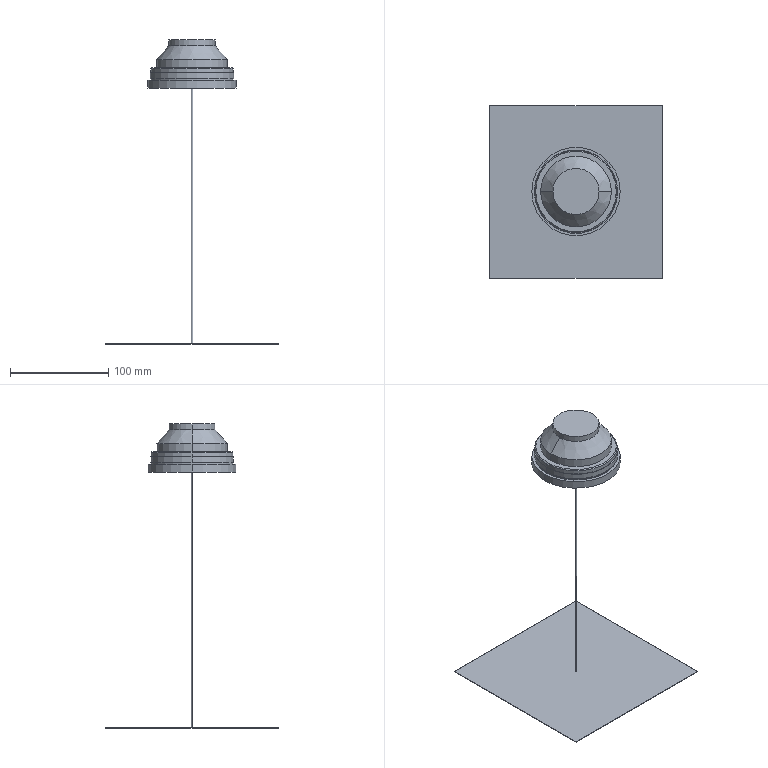Part | SolidWorks | features ICE 8, Draft 3, Chamfer 2, Extrusion 1, RevCut 1 | 1 solid | 30 faces | box 175 x 175 x 309.5 mm | volume 221478 mm3 | cylinder 14 | plane 12 | cone 4 | commonest cylinder face diameters 84 x4 2 x2 47 x2 72 x2 85 x2 90 x2
STEP:
#1=CARTESIAN_POINT('',(-1.,0.,-260.));
#2=VERTEX_POINT('',#1);
#3=CARTESIAN_POINT('',(1.,0.,-260.));
#4=VERTEX_POINT('',#3);
#5=CARTESIAN_POINT('',(0.,0.,-260.));
#6=DIRECTION('',(0.,0.,-1.));
#7=DIRECTION('',(-1.,0.,0.));
#8=AXIS2_PLACEMENT_3D('',#5,#6,#7);
#9=CIRCLE('',#8,1.);
#10=EDGE_CURVE('',#2,#4,#9,.T.);
#11=ORIENTED_EDGE('',*,*,#10,.F.);
#12=CARTESIAN_POINT('',(-1.,0.,0.));
#13=VERTEX_POINT('',#12);
#14=CARTESIAN_POINT('',(-1.,0.,-260.));
#15=DIRECTION('',(0.,0.,1.));
#16=VECTOR('',#15,1000.);
#17=LINE('',#14,#16);
#18=EDGE_CURVE('',#2,#13,#17,.T.);
#19=ORIENTED_EDGE('',*,*,#18,.T.);
#20=CARTESIAN_POINT('',(1.,0.,0.));
#21=VERTEX_POINT('',#20);
#22=CARTESIAN_POINT('',(0.,0.,0.));
#23=DIRECTION('',(0.,0.,-1.));
#24=DIRECTION('',(1.,0.,0.));
#25=AXIS2_PLACEMENT_3D('',#22,#23,#24);
#26=CIRCLE('',#25,1.);
#27=EDGE_CURVE('',#13,#21,#26,.T.);
#28=ORIENTED_EDGE('',*,*,#27,.T.);
#29=CARTESIAN_POINT('',(1.,0.,-260.));
#30=DIRECTION('',(0.,0.,1.));
#31=VECTOR('',#30,1000.);
#32=LINE('',#29,#31);
#33=EDGE_CURVE('',#4,#21,#32,.T.);
#34=ORIENTED_EDGE('',*,*,#33,.F.);
#35=EDGE_LOOP('',(#11,#19,#28,#34));
#36=FACE_OUTER_BOUND('',#35,.T.);
#37=CARTESIAN_POINT('',(0.,0.,-260.));
#38=DIRECTION('',(0.,0.,1.));
#39=DIRECTION('',(1.,0.,0.));
#40=AXIS2_PLACEMENT_3D('',#37,#38,#39);
#41=CYLINDRICAL_SURFACE('',#40,1.);
#42=ADVANCED_FACE('',(#36),#41,.T.);
#43=CARTESIAN_POINT('',(41.,0.,20.5));
#44=VERTEX_POINT('',#43);
#45=CARTESIAN_POINT('',(-41.,0.,20.5));
#46=VERTEX_POINT('',#45);
#47=CARTESIAN_POINT('',(0.,0.,20.5));
#48=DIRECTION('',(0.,0.,1.));
#49=DIRECTION('',(1.,0.,0.));
#50=AXIS2_PLACEMENT_3D('',#47,#48,#49);
#51=CIRCLE('',#50,41.);
#52=EDGE_CURVE('',#44,#46,#51,.T.);
#53=ORIENTED_EDGE('',*,*,#52,.F.);
#54=CARTESIAN_POINT('',(42.,0.,19.5));
#55=VERTEX_POINT('',#54);
#56=CARTESIAN_POINT('',(42.,0.,19.5));
#57=DIRECTION('',(0.7071,0.,-0.7071));
#58=VECTOR('',#57,1000.);
#59=LINE('',#56,#58);
#60=EDGE_CURVE('',#44,#55,#59,.T.);
#61=ORIENTED_EDGE('',*,*,#60,.T.);
#62=CARTESIAN_POINT('',(-42.,0.,19.5));
#63=VERTEX_POINT('',#62);
#64=CARTESIAN_POINT('',(0.,0.,19.5));
#65=DIRECTION('',(0.,0.,-1.));
#66=DIRECTION('',(1.,0.,0.));
#67=AXIS2_PLACEMENT_3D('',#64,#65,#66);
#68=CIRCLE('',#67,42.);
#69=EDGE_CURVE('',#63,#55,#68,.T.);
#70=ORIENTED_EDGE('',*,*,#69,.F.);
#71=CARTESIAN_POINT('',(-42.,0.,19.5));
#72=DIRECTION('',(-0.7071,0.,-0.7071));
#73=VECTOR('',#72,1000.);
#74=LINE('',#71,#73);
#75=EDGE_CURVE('',#46,#63,#74,.T.);
#76=ORIENTED_EDGE('',*,*,#75,.F.);
#77=EDGE_LOOP('',(#53,#61,#70,#76));
#78=FACE_OUTER_BOUND('',#77,.T.);
#79=CARTESIAN_POINT('',(0.,0.,19.5));
#80=DIRECTION('',(0.,0.,-1.));
#81=DIRECTION('',(-1.,0.,0.));
#82=AXIS2_PLACEMENT_3D('',#79,#80,#81);
#83=CONICAL_SURFACE('',#82,42.,0.7854);
#84=ADVANCED_FACE('',(#78),#83,.T.);
#85=CARTESIAN_POINT('',(36.,0.,29.));
#86=VERTEX_POINT('',#85);
#87=CARTESIAN_POINT('',(-36.,0.,29.));
#88=VERTEX_POINT('',#87);
#89=CARTESIAN_POINT('',(0.,0.,29.));
#90=DIRECTION('',(0.,0.,1.));
#91=DIRECTION('',(1.,0.,0.));
#92=AXIS2_PLACEMENT_3D('',#89,#90,#91);
#93=CIRCLE('',#92,36.);
#94=EDGE_CURVE('',#86,#88,#93,.T.);
#95=ORIENTED_EDGE('',*,*,#94,.F.);
#96=CARTESIAN_POINT('',(36.,0.,20.5));
#97=VERTEX_POINT('',#96);
#98=CARTESIAN_POINT('',(36.,0.,29.));
#99=DIRECTION('',(0.,0.,-1.));
#100=VECTOR('',#99,1000.);
#101=LINE('',#98,#100);
#102=EDGE_CURVE('',#86,#97,#101,.T.);
#103=ORIENTED_EDGE('',*,*,#102,.T.);
#104=CARTESIAN_POINT('',(-36.,0.,20.5));
#105=VERTEX_POINT('',#104);
#106=CARTESIAN_POINT('',(0.,0.,20.5));
#107=DIRECTION('',(0.,0.,1.));
#108=DIRECTION('',(1.,0.,0.));
#109=AXIS2_PLACEMENT_3D('',#106,#107,#108);
#110=CIRCLE('',#109,36.);
#111=EDGE_CURVE('',#97,#105,#110,.T.);
#112=ORIENTED_EDGE('',*,*,#111,.T.);
#113=CARTESIAN_POINT('',(-36.,0.,29.));
#114=DIRECTION('',(0.,0.,-1.));
#115=VECTOR('',#114,1000.);
#116=LINE('',#113,#115);
#117=EDGE_CURVE('',#88,#105,#116,.T.);
#118=ORIENTED_EDGE('',*,*,#117,.F.);
#119=EDGE_LOOP('',(#95,#103,#112,#118));
#120=FACE_OUTER_BOUND('',#119,.T.);
#121=CARTESIAN_POINT('',(0.,0.,29.));
#122=DIRECTION('',(0.,0.,-1.));
#123=DIRECTION('',(-1.,0.,0.));
#124=AXIS2_PLACEMENT_3D('',#121,#122,#123);
#125=CYLINDRICAL_SURFACE('',#124,36.);
#126=ADVANCED_FACE('',(#120),#125,.T.);
#127=CARTESIAN_POINT('',(23.5,0.,43.));
#128=VERTEX_POINT('',#127);
#129=CARTESIAN_POINT('',(-23.5,0.,43.));
#130=VERTEX_POINT('',#129);
#131=CARTESIAN_POINT('',(0.,0.,43.));
#132=DIRECTION('',(0.,0.,1.));
#133=DIRECTION('',(1.,0.,0.));
#134=AXIS2_PLACEMENT_3D('',#131,#132,#133);
#135=CIRCLE('',#134,23.5);
#136=EDGE_CURVE('',#128,#130,#135,.T.);
#137=ORIENTED_EDGE('',*,*,#136,.F.);
#138=CARTESIAN_POINT('',(23.5,0.,43.));
#139=DIRECTION('',(0.666,0.,-0.7459));
#140=VECTOR('',#139,1000.);
#141=LINE('',#138,#140);
#142=EDGE_CURVE('',#128,#86,#141,.T.);
#143=ORIENTED_EDGE('',*,*,#142,.T.);
#144=ORIENTED_EDGE('',*,*,#94,.T.);
#145=CARTESIAN_POINT('',(-23.5,0.,43.));
#146=DIRECTION('',(-0.666,0.,-0.7459));
#147=VECTOR('',#146,1000.);
#148=LINE('',#145,#147);
#149=EDGE_CURVE('',#130,#88,#148,.T.);
#150=ORIENTED_EDGE('',*,*,#149,.F.);
#151=EDGE_LOOP('',(#137,#143,#144,#150));
#152=FACE_OUTER_BOUND('',#151,.T.);
#153=CARTESIAN_POINT('',(0.,0.,43.));
#154=DIRECTION('',(0.,0.,-1.));
#155=DIRECTION('',(-1.,0.,0.));
#156=AXIS2_PLACEMENT_3D('',#153,#154,#155);
#157=CONICAL_SURFACE('',#156,23.5,0.7289);
#158=ADVANCED_FACE('',(#152),#157,.T.);
#159=CARTESIAN_POINT('',(23.5,0.,49.));
#160=VERTEX_POINT('',#159);
#161=CARTESIAN_POINT('',(-23.5,0.,49.));
#162=VERTEX_POINT('',#161);
#163=CARTESIAN_POINT('',(0.,0.,49.));
#164=DIRECTION('',(0.,0.,1.));
#165=DIRECTION('',(1.,0.,0.));
#166=AXIS2_PLACEMENT_3D('',#163,#164,#165);
#167=CIRCLE('',#166,23.5);
#168=EDGE_CURVE('',#160,#162,#167,.T.);
#169=ORIENTED_EDGE('',*,*,#168,.F.);
#170=CARTESIAN_POINT('',(23.5,0.,49.));
#171=DIRECTION('',(0.,0.,-1.));
#172=VECTOR('',#171,1000.);
#173=LINE('',#170,#172);
#174=EDGE_CURVE('',#160,#128,#173,.T.);
#175=ORIENTED_EDGE('',*,*,#174,.T.);
#176=ORIENTED_EDGE('',*,*,#136,.T.);
#177=CARTESIAN_POINT('',(-23.5,0.,49.));
#178=DIRECTION('',(0.,0.,-1.));
#179=VECTOR('',#178,1000.);
#180=LINE('',#177,#179);
#181=EDGE_CURVE('',#162,#130,#180,.T.);
#182=ORIENTED_EDGE('',*,*,#181,.F.);
#183=EDGE_LOOP('',(#169,#175,#176,#182));
#184=FACE_OUTER_BOUND('',#183,.T.);
#185=CARTESIAN_POINT('',(0.,0.,49.));
#186=DIRECTION('',(0.,0.,-1.));
#187=DIRECTION('',(-1.,0.,0.));
#188=AXIS2_PLACEMENT_3D('',#185,#186,#187);
#189=CYLINDRICAL_SURFACE('',#188,23.5);
#190=ADVANCED_FACE('',(#184),#189,.T.);
#191=ORIENTED_EDGE('',*,*,#69,.T.);
#192=CARTESIAN_POINT('',(42.,0.,15.5));
#193=VERTEX_POINT('',#192);
#194=CARTESIAN_POINT('',(42.,0.,0.));
#195=DIRECTION('',(0.,0.,-1.));
#196=VECTOR('',#195,1000.);
#197=LINE('',#194,#196);
#198=EDGE_CURVE('',#55,#193,#197,.T.);
#199=ORIENTED_EDGE('',*,*,#198,.T.);
#200=CARTESIAN_POINT('',(-42.,0.,15.5));
#201=VERTEX_POINT('',#200);
#202=CARTESIAN_POINT('',(0.,0.,15.5));
#203=DIRECTION('',(0.,0.,-1.));
#204=DIRECTION('',(-1.,0.,0.));
#205=AXIS2_PLACEMENT_3D('',#202,#203,#204);
#206=CIRCLE('',#205,42.);
#207=EDGE_CURVE('',#201,#193,#206,.T.);
#208=ORIENTED_EDGE('',*,*,#207,.F.);
#209=CARTESIAN_POINT('',(-42.,0.,0.));
#210=DIRECTION('',(0.,0.,-1.));
#211=VECTOR('',#210,1000.);
#212=LINE('',#209,#211);
#213=EDGE_CURVE('',#63,#201,#212,.T.);
#214=ORIENTED_EDGE('',*,*,#213,.F.);
#215=EDGE_LOOP('',(#191,#199,#208,#214));
#216=FACE_OUTER_BOUND('',#215,.T.);
#217=CARTESIAN_POINT('',(0.,0.,0.));
#218=DIRECTION('',(0.,0.,-1.));
#219=DIRECTION('',(-1.,0.,0.));
#220=AXIS2_PLACEMENT_3D('',#217,#218,#219);
#221=CYLINDRICAL_SURFACE('',#220,42.);
#222=ADVANCED_FACE('',(#216),#221,.T.);
#223=CARTESIAN_POINT('',(45.,0.,8.));
#224=VERTEX_POINT('',#223);
#225=CARTESIAN_POINT('',(-45.,0.,8.));
#226=VERTEX_POINT('',#225);
#227=CARTESIAN_POINT('',(0.,0.,8.));
#228=DIRECTION('',(0.,0.,1.));
#229=DIRECTION('',(1.,0.,0.));
#230=AXIS2_PLACEMENT_3D('',#227,#228,#229);
#231=CIRCLE('',#230,45.);
#232=EDGE_CURVE('',#224,#226,#231,.T.);
#233=ORIENTED_EDGE('',*,*,#232,.F.);
#234=CARTESIAN_POINT('',(45.,0.,0.));
#235=VERTEX_POINT('',#234);
#236=CARTESIAN_POINT('',(45.,0.,8.));
#237=DIRECTION('',(0.,0.,-1.));
#238=VECTOR('',#237,1000.);
#239=LINE('',#236,#238);
#240=EDGE_CURVE('',#224,#235,#239,.T.);
#241=ORIENTED_EDGE('',*,*,#240,.T.);
#242=CARTESIAN_POINT('',(-45.,0.,0.));
#243=VERTEX_POINT('',#242);
#244=CARTESIAN_POINT('',(0.,0.,0.));
#245=DIRECTION('',(0.,0.,1.));
#246=DIRECTION('',(1.,0.,0.));
#247=AXIS2_PLACEMENT_3D('',#244,#245,#246);
#248=CIRCLE('',#247,45.);
#249=EDGE_CURVE('',#235,#243,#248,.T.);
#250=ORIENTED_EDGE('',*,*,#249,.T.);
#251=CARTESIAN_POINT('',(-45.,0.,8.));
#252=DIRECTION('',(0.,0.,-1.));
#253=VECTOR('',#252,1000.);
#254=LINE('',#251,#253);
#255=EDGE_CURVE('',#226,#243,#254,.T.);
#256=ORIENTED_EDGE('',*,*,#255,.F.);
#257=EDGE_LOOP('',(#233,#241,#250,#256));
#258=FACE_OUTER_BOUND('',#257,.T.);
#259=CARTESIAN_POINT('',(0.,0.,8.));
#260=DIRECTION('',(0.,0.,-1.));
#261=DIRECTION('',(-1.,0.,0.));
#262=AXIS2_PLACEMENT_3D('',#259,#260,#261);
#263=CYLINDRICAL_SURFACE('',#262,45.);
#264=ADVANCED_FACE('',(#258),#263,.T.);
#265=CARTESIAN_POINT('',(-42.,0.,9.5));
#266=VERTEX_POINT('',#265);
#267=CARTESIAN_POINT('',(42.,0.,9.5));
#268=VERTEX_POINT('',#267);
#269=CARTESIAN_POINT('',(0.,0.,9.5));
#270=DIRECTION('',(0.,0.,-1.));
#271=DIRECTION('',(-1.,0.,0.));
#272=AXIS2_PLACEMENT_3D('',#269,#270,#271);
#273=CIRCLE('',#272,42.);
#274=EDGE_CURVE('',#266,#268,#273,.T.);
#275=ORIENTED_EDGE('',*,*,#274,.T.);
#276=CARTESIAN_POINT('',(42.,0.,8.));
#277=VERTEX_POINT('',#276);
#278=CARTESIAN_POINT('',(42.,0.,0.));
#279=DIRECTION('',(0.,0.,-1.));
#280=VECTOR('',#279,1000.);
#281=LINE('',#278,#280);
#282=EDGE_CURVE('',#268,#277,#281,.T.);
#283=ORIENTED_EDGE('',*,*,#282,.T.);
#284=CARTESIAN_POINT('',(-42.,0.,8.));
#285=VERTEX_POINT('',#284);
#286=CARTESIAN_POINT('',(0.,0.,8.));
#287=DIRECTION('',(0.,0.,-1.));
#288=DIRECTION('',(-1.,0.,0.));
#289=AXIS2_PLACEMENT_3D('',#286,#287,#288);
#290=CIRCLE('',#289,42.);
#291=EDGE_CURVE('',#285,#277,#290,.T.);
#292=ORIENTED_EDGE('',*,*,#291,.F.);
#293=CARTESIAN_POINT('',(-42.,0.,0.));
#294=DIRECTION('',(0.,0.,-1.));
#295=VECTOR('',#294,1000.);
#296=LINE('',#293,#295);
#297=EDGE_CURVE('',#266,#285,#296,.T.);
#298=ORIENTED_EDGE('',*,*,#297,.F.);
#299=EDGE_LOOP('',(#275,#283,#292,#298));
#300=FACE_OUTER_BOUND('',#299,.T.);
#301=CARTESIAN_POINT('',(0.,0.,0.));
#302=DIRECTION('',(0.,0.,-1.));
#303=DIRECTION('',(-1.,0.,0.));
#304=AXIS2_PLACEMENT_3D('',#301,#302,#303);
#305=CYLINDRICAL_SURFACE('',#304,42.);
#306=ADVANCED_FACE('',(#300),#305,.T.);
#307=CARTESIAN_POINT('',(-42.5,0.,15.5));
#308=VERTEX_POINT('',#307);
#309=CARTESIAN_POINT('',(42.5,0.,15.5));
#310=VERTEX_POINT('',#309);
#311=CARTESIAN_POINT('',(0.,0.,15.5));
#312=DIRECTION('',(0.,0.,-1.));
#313=DIRECTION('',(-1.,0.,0.));
#314=AXIS2_PLACEMENT_3D('',#311,#312,#313);
#315=CIRCLE('',#314,42.5);
#316=EDGE_CURVE('',#308,#310,#315,.T.);
#317=ORIENTED_EDGE('',*,*,#316,.T.);
#318=CARTESIAN_POINT('',(42.5,0.,9.5));
#319=VERTEX_POINT('',#318);
#320=CARTESIAN_POINT('',(42.5,0.,20.5));
#321=DIRECTION('',(0.,0.,-1.));
#322=VECTOR('',#321,1000.);
#323=LINE('',#320,#322);
#324=EDGE_CURVE('',#310,#319,#323,.T.);
#325=ORIENTED_EDGE('',*,*,#324,.T.);
#326=CARTESIAN_POINT('',(-42.5,0.,9.5));
#327=VERTEX_POINT('',#326);
#328=CARTESIAN_POINT('',(0.,0.,9.5));
#329=DIRECTION('',(0.,0.,-1.));
#330=DIRECTION('',(-1.,0.,0.));
#331=AXIS2_PLACEMENT_3D('',#328,#329,#330);
#332=CIRCLE('',#331,42.5);
#333=EDGE_CURVE('',#327,#319,#332,.T.);
#334=ORIENTED_EDGE('',*,*,#333,.F.);
#335=CARTESIAN_POINT('',(-42.5,0.,20.5));
#336=DIRECTION('',(0.,0.,-1.));
#337=VECTOR('',#336,1000.);
#338=LINE('',#335,#337);
#339=EDGE_CURVE('',#308,#327,#338,.T.);
#340=ORIENTED_EDGE('',*,*,#339,.F.);
#341=EDGE_LOOP('',(#317,#325,#334,#340));
#342=FACE_OUTER_BOUND('',#341,.T.);
#343=CARTESIAN_POINT('',(0.,0.,20.5));
#344=DIRECTION('',(0.,0.,-1.));
#345=DIRECTION('',(-1.,0.,0.));
#346=AXIS2_PLACEMENT_3D('',#343,#344,#345);
#347=CYLINDRICAL_SURFACE('',#346,42.5);
#348=ADVANCED_FACE('',(#342),#347,.T.);
#349=ORIENTED_EDGE('',*,*,#324,.F.);
#350=CARTESIAN_POINT('',(0.,0.,15.5));
#351=DIRECTION('',(0.,0.,-1.));
#352=DIRECTION('',(-1.,0.,0.));
#353=AXIS2_PLACEMENT_3D('',#350,#351,#352);
#354=CIRCLE('',#353,42.5);
#355=EDGE_CURVE('',#310,#308,#354,.T.);
#356=ORIENTED_EDGE('',*,*,#355,.T.);
#357=ORIENTED_EDGE('',*,*,#339,.T.);
#358=CARTESIAN_POINT('',(0.,0.,9.5));
#359=DIRECTION('',(0.,0.,-1.));
#360=DIRECTION('',(-1.,0.,0.));
#361=AXIS2_PLACEMENT_3D('',#358,#359,#360);
#362=CIRCLE('',#361,42.5);
#363=EDGE_CURVE('',#319,#327,#362,.T.);
#364=ORIENTED_EDGE('',*,*,#363,.F.);
#365=EDGE_LOOP('',(#349,#356,#357,#364));
#366=FACE_OUTER_BOUND('',#365,.T.);
#367=CARTESIAN_POINT('',(0.,0.,20.5));
#368=DIRECTION('',(0.,0.,-1.));
#369=DIRECTION('',(-1.,0.,0.));
#370=AXIS2_PLACEMENT_3D('',#367,#368,#369);
#371=CYLINDRICAL_SURFACE('',#370,42.5);
#372=ADVANCED_FACE('',(#366),#371,.T.);
#373=ORIENTED_EDGE('',*,*,#282,.F.);
#374=CARTESIAN_POINT('',(0.,0.,9.5));
#375=DIRECTION('',(0.,0.,-1.));
#376=DIRECTION('',(-1.,0.,0.));
#377=AXIS2_PLACEMENT_3D('',#374,#375,#376);
#378=CIRCLE('',#377,42.);
#379=EDGE_CURVE('',#268,#266,#378,.T.);
#380=ORIENTED_EDGE('',*,*,#379,.T.);
#381=ORIENTED_EDGE('',*,*,#297,.T.);
#382=CARTESIAN_POINT('',(0.,0.,8.));
#383=DIRECTION('',(0.,0.,-1.));
#384=DIRECTION('',(-1.,0.,0.));
#385=AXIS2_PLACEMENT_3D('',#382,#383,#384);
#386=CIRCLE('',#385,42.);
#387=EDGE_CURVE('',#277,#285,#386,.T.);
#388=ORIENTED_EDGE('',*,*,#387,.F.);
#389=EDGE_LOOP('',(#373,#380,#381,#388));
#390=FACE_OUTER_BOUND('',#389,.T.);
#391=CARTESIAN_POINT('',(0.,0.,0.));
#392=DIRECTION('',(0.,0.,-1.));
#393=DIRECTION('',(-1.,0.,0.));
#394=AXIS2_PLACEMENT_3D('',#391,#392,#393);
#395=CYLINDRICAL_SURFACE('',#394,42.);
#396=ADVANCED_FACE('',(#390),#395,.T.);
#397=ORIENTED_EDGE('',*,*,#274,.F.);
#398=ORIENTED_EDGE('',*,*,#379,.F.);
#399=EDGE_LOOP('',(#397,#398));
#400=FACE_BOUND('',#399,.T.);
#401=ORIENTED_EDGE('',*,*,#333,.T.);
#402=ORIENTED_EDGE('',*,*,#363,.T.);
#403=EDGE_LOOP('',(#401,#402));
#404=FACE_OUTER_BOUND('',#403,.T.);
#405=CARTESIAN_POINT('',(-42.,0.,9.5));
#406=DIRECTION('',(0.,0.,1.));
#407=DIRECTION('',(1.,0.,0.));
#408=AXIS2_PLACEMENT_3D('',#405,#406,#407);
#409=PLANE('',#408);
#410=ADVANCED_FACE('',(#400,#404),#409,.F.);
#411=CARTESIAN_POINT('',(0.,0.,0.));
#412=DIRECTION('',(0.,0.,-1.));
#413=DIRECTION('',(1.,0.,0.));
#414=AXIS2_PLACEMENT_3D('',#411,#412,#413);
#415=CIRCLE('',#414,1.);
#416=EDGE_CURVE('',#21,#13,#415,.T.);
#417=ORIENTED_EDGE('',*,*,#416,.F.);
#418=ORIENTED_EDGE('',*,*,#27,.F.);
#419=EDGE_LOOP('',(#417,#418));
#420=FACE_BOUND('',#419,.T.);
#421=CARTESIAN_POINT('',(0.,0.,0.));
#422=DIRECTION('',(0.,0.,1.));
#423=DIRECTION('',(1.,0.,0.));
#424=AXIS2_PLACEMENT_3D('',#421,#422,#423);
#425=CIRCLE('',#424,45.);
#426=EDGE_CURVE('',#243,#235,#425,.T.);
#427=ORIENTED_EDGE('',*,*,#426,.F.);
#428=ORIENTED_EDGE('',*,*,#249,.F.);
#429=EDGE_LOOP('',(#427,#428));
#430=FACE_OUTER_BOUND('',#429,.T.);
#431=CARTESIAN_POINT('',(0.,0.,0.));
#432=DIRECTION('',(0.,0.,1.));
#433=DIRECTION('',(1.,0.,0.));
#434=AXIS2_PLACEMENT_3D('',#431,#432,#433);
#435=PLANE('',#434);
#436=ADVANCED_FACE('',(#420,#430),#435,.F.);
#437=ORIENTED_EDGE('',*,*,#240,.F.);
#438=CARTESIAN_POINT('',(0.,0.,8.));
#439=DIRECTION('',(0.,0.,1.));
#440=DIRECTION('',(1.,0.,0.));
#441=AXIS2_PLACEMENT_3D('',#438,#439,#440);
#442=CIRCLE('',#441,45.);
#443=EDGE_CURVE('',#226,#224,#442,.T.);
#444=ORIENTED_EDGE('',*,*,#443,.F.);
#445=ORIENTED_EDGE('',*,*,#255,.T.);
#446=ORIENTED_EDGE('',*,*,#426,.T.);
#447=EDGE_LOOP('',(#437,#444,#445,#446));
#448=FACE_OUTER_BOUND('',#447,.T.);
#449=CARTESIAN_POINT('',(0.,0.,8.));
#450=DIRECTION('',(0.,0.,-1.));
#451=DIRECTION('',(-1.,0.,0.));
#452=AXIS2_PLACEMENT_3D('',#449,#450,#451);
#453=CYLINDRICAL_SURFACE('',#452,45.);
#454=ADVANCED_FACE('',(#448),#453,.T.);
#455=ORIENTED_EDGE('',*,*,#443,.T.);
#456=ORIENTED_EDGE('',*,*,#232,.T.);
#457=EDGE_LOOP('',(#455,#456));
#458=FACE_OUTER_BOUND('',#457,.T.);
#459=ORIENTED_EDGE('',*,*,#291,.T.);
#460=ORIENTED_EDGE('',*,*,#387,.T.);
#461=EDGE_LOOP('',(#459,#460));
#462=FACE_BOUND('',#461,.T.);
#463=CARTESIAN_POINT('',(0.,0.,8.));
#464=DIRECTION('',(0.,0.,1.));
#465=DIRECTION('',(1.,0.,0.));
#466=AXIS2_PLACEMENT_3D('',#463,#464,#465);
#467=PLANE('',#466);
#468=ADVANCED_FACE('',(#458,#462),#467,.T.);
#469=ORIENTED_EDGE('',*,*,#198,.F.);
#470=CARTESIAN_POINT('',(0.,0.,19.5));
#471=DIRECTION('',(0.,0.,-1.));
#472=DIRECTION('',(1.,0.,0.));
#473=AXIS2_PLACEMENT_3D('',#470,#471,#472);
#474=CIRCLE('',#473,42.);
#475=EDGE_CURVE('',#55,#63,#474,.T.);
#476=ORIENTED_EDGE('',*,*,#475,.T.);
#477=ORIENTED_EDGE('',*,*,#213,.T.);
#478=CARTESIAN_POINT('',(0.,0.,15.5));
#479=DIRECTION('',(0.,0.,-1.));
#480=DIRECTION('',(-1.,0.,0.));
#481=AXIS2_PLACEMENT_3D('',#478,#479,#480);
#482=CIRCLE('',#481,42.);
#483=EDGE_CURVE('',#193,#201,#482,.T.);
#484=ORIENTED_EDGE('',*,*,#483,.F.);
#485=EDGE_LOOP('',(#469,#476,#477,#484));
#486=FACE_OUTER_BOUND('',#485,.T.);
#487=CARTESIAN_POINT('',(0.,0.,0.));
#488=DIRECTION('',(0.,0.,-1.));
#489=DIRECTION('',(-1.,0.,0.));
#490=AXIS2_PLACEMENT_3D('',#487,#488,#489);
#491=CYLINDRICAL_SURFACE('',#490,42.);
#492=ADVANCED_FACE('',(#486),#491,.T.);
#493=ORIENTED_EDGE('',*,*,#316,.F.);
#494=ORIENTED_EDGE('',*,*,#355,.F.);
#495=EDGE_LOOP('',(#493,#494));
#496=FACE_OUTER_BOUND('',#495,.T.);
#497=ORIENTED_EDGE('',*,*,#207,.T.);
#498=ORIENTED_EDGE('',*,*,#483,.T.);
#499=EDGE_LOOP('',(#497,#498));
#500=FACE_BOUND('',#499,.T.);
#501=CARTESIAN_POINT('',(-42.,0.,15.5));
#502=DIRECTION('',(0.,0.,-1.));
#503=DIRECTION('',(-1.,0.,0.));
#504=AXIS2_PLACEMENT_3D('',#501,#502,#503);
#505=PLANE('',#504);
#506=ADVANCED_FACE('',(#496,#500),#505,.F.);
#507=CARTESIAN_POINT('',(0.,0.,49.));
#508=DIRECTION('',(0.,0.,1.));
#509=DIRECTION('',(1.,0.,0.));
#510=AXIS2_PLACEMENT_3D('',#507,#508,#509);
#511=CIRCLE('',#510,23.5);
#512=EDGE_CURVE('',#162,#160,#511,.T.);
#513=ORIENTED_EDGE('',*,*,#512,.T.);
#514=ORIENTED_EDGE('',*,*,#168,.T.);
#515=EDGE_LOOP('',(#513,#514));
#516=FACE_OUTER_BOUND('',#515,.T.);
#517=CARTESIAN_POINT('',(0.,0.,49.));
#518=DIRECTION('',(0.,0.,1.));
#519=DIRECTION('',(1.,0.,0.));
#520=AXIS2_PLACEMENT_3D('',#517,#518,#519);
#521=PLANE('',#520);
#522=ADVANCED_FACE('',(#516),#521,.T.);
#523=ORIENTED_EDGE('',*,*,#174,.F.);
#524=ORIENTED_EDGE('',*,*,#512,.F.);
#525=ORIENTED_EDGE('',*,*,#181,.T.);
#526=CARTESIAN_POINT('',(0.,0.,43.));
#527=DIRECTION('',(0.,0.,1.));
#528=DIRECTION('',(1.,0.,0.));
#529=AXIS2_PLACEMENT_3D('',#526,#527,#528);
#530=CIRCLE('',#529,23.5);
#531=EDGE_CURVE('',#130,#128,#530,.T.);
#532=ORIENTED_EDGE('',*,*,#531,.T.);
#533=EDGE_LOOP('',(#523,#524,#525,#532));
#534=FACE_OUTER_BOUND('',#533,.T.);
#535=CARTESIAN_POINT('',(0.,0.,49.));
#536=DIRECTION('',(0.,0.,-1.));
#537=DIRECTION('',(-1.,0.,0.));
#538=AXIS2_PLACEMENT_3D('',#535,#536,#537);
#539=CYLINDRICAL_SURFACE('',#538,23.5);
#540=ADVANCED_FACE('',(#534),#539,.T.);
#541=ORIENTED_EDGE('',*,*,#142,.F.);
#542=ORIENTED_EDGE('',*,*,#531,.F.);
#543=ORIENTED_EDGE('',*,*,#149,.T.);
#544=CARTESIAN_POINT('',(0.,0.,29.));
#545=DIRECTION('',(0.,0.,1.));
#546=DIRECTION('',(1.,0.,0.));
#547=AXIS2_PLACEMENT_3D('',#544,#545,#546);
#548=CIRCLE('',#547,36.);
#549=EDGE_CURVE('',#88,#86,#548,.T.);
#550=ORIENTED_EDGE('',*,*,#549,.T.);
#551=EDGE_LOOP('',(#541,#542,#543,#550));
#552=FACE_OUTER_BOUND('',#551,.T.);
#553=CARTESIAN_POINT('',(0.,0.,43.));
#554=DIRECTION('',(0.,0.,-1.));
#555=DIRECTION('',(-1.,0.,0.));
#556=AXIS2_PLACEMENT_3D('',#553,#554,#555);
#557=CONICAL_SURFACE('',#556,23.5,0.7289);
#558=ADVANCED_FACE('',(#552),#557,.T.);
#559=ORIENTED_EDGE('',*,*,#102,.F.);
#560=ORIENTED_EDGE('',*,*,#549,.F.);
#561=ORIENTED_EDGE('',*,*,#117,.T.);
#562=CARTESIAN_POINT('',(0.,0.,20.5));
#563=DIRECTION('',(0.,0.,1.));
#564=DIRECTION('',(1.,0.,0.));
#565=AXIS2_PLACEMENT_3D('',#562,#563,#564);
#566=CIRCLE('',#565,36.);
#567=EDGE_CURVE('',#105,#97,#566,.T.);
#568=ORIENTED_EDGE('',*,*,#567,.T.);
#569=EDGE_LOOP('',(#559,#560,#561,#568));
#570=FACE_OUTER_BOUND('',#569,.T.);
#571=CARTESIAN_POINT('',(0.,0.,29.));
#572=DIRECTION('',(0.,0.,-1.));
#573=DIRECTION('',(-1.,0.,0.));
#574=AXIS2_PLACEMENT_3D('',#571,#572,#573);
#575=CYLINDRICAL_SURFACE('',#574,36.);
#576=ADVANCED_FACE('',(#570),#575,.T.);
#577=CARTESIAN_POINT('',(0.,0.,20.5));
#578=DIRECTION('',(0.,0.,1.));
#579=DIRECTION('',(1.,0.,0.));
#580=AXIS2_PLACEMENT_3D('',#577,#578,#579);
#581=CIRCLE('',#580,41.);
#582=EDGE_CURVE('',#46,#44,#581,.T.);
#583=ORIENTED_EDGE('',*,*,#582,.T.);
#584=ORIENTED_EDGE('',*,*,#52,.T.);
#585=EDGE_LOOP('',(#583,#584));
#586=FACE_OUTER_BOUND('',#585,.T.);
#587=ORIENTED_EDGE('',*,*,#567,.F.);
#588=ORIENTED_EDGE('',*,*,#111,.F.);
#589=EDGE_LOOP('',(#587,#588));
#590=FACE_BOUND('',#589,.T.);
#591=CARTESIAN_POINT('',(0.,0.,20.5));
#592=DIRECTION('',(0.,0.,1.));
#593=DIRECTION('',(1.,0.,0.));
#594=AXIS2_PLACEMENT_3D('',#591,#592,#593);
#595=PLANE('',#594);
#596=ADVANCED_FACE('',(#586,#590),#595,.T.);
#597=ORIENTED_EDGE('',*,*,#60,.F.);
#598=ORIENTED_EDGE('',*,*,#582,.F.);
#599=ORIENTED_EDGE('',*,*,#75,.T.);
#600=ORIENTED_EDGE('',*,*,#475,.F.);
#601=EDGE_LOOP('',(#597,#598,#599,#600));
#602=FACE_OUTER_BOUND('',#601,.T.);
#603=CARTESIAN_POINT('',(0.,0.,19.5));
#604=DIRECTION('',(0.,0.,-1.));
#605=DIRECTION('',(-1.,0.,0.));
#606=AXIS2_PLACEMENT_3D('',#603,#604,#605);
#607=CONICAL_SURFACE('',#606,42.,0.7854);
#608=ADVANCED_FACE('',(#602),#607,.T.);
#609=ORIENTED_EDGE('',*,*,#18,.F.);
#610=CARTESIAN_POINT('',(0.,0.,-260.));
#611=DIRECTION('',(0.,0.,-1.));
#612=DIRECTION('',(-1.,0.,0.));
#613=AXIS2_PLACEMENT_3D('',#610,#611,#612);
#614=CIRCLE('',#613,1.);
#615=EDGE_CURVE('',#4,#2,#614,.T.);
#616=ORIENTED_EDGE('',*,*,#615,.F.);
#617=ORIENTED_EDGE('',*,*,#33,.T.);
#618=ORIENTED_EDGE('',*,*,#416,.T.);
#619=EDGE_LOOP('',(#609,#616,#617,#618));
#620=FACE_OUTER_BOUND('',#619,.T.);
#621=CARTESIAN_POINT('',(0.,0.,-260.));
#622=DIRECTION('',(0.,0.,1.));
#623=DIRECTION('',(1.,0.,0.));
#624=AXIS2_PLACEMENT_3D('',#621,#622,#623);
#625=CYLINDRICAL_SURFACE('',#624,1.);
#626=ADVANCED_FACE('',(#620),#625,.T.);
#627=CARTESIAN_POINT('',(-87.5,-87.5,-260.));
#628=VERTEX_POINT('',#627);
#629=CARTESIAN_POINT('',(-87.5,87.5,-260.));
#630=VERTEX_POINT('',#629);
#631=CARTESIAN_POINT('',(-87.5,87.5,-260.));
#632=DIRECTION('',(0.,1.,0.));
#633=VECTOR('',#632,1000.);
#634=LINE('',#631,#633);
#635=EDGE_CURVE('',#628,#630,#634,.T.);
#636=ORIENTED_EDGE('',*,*,#635,.T.);
#637=CARTESIAN_POINT('',(-87.5,87.5,-260.5));
#638=VERTEX_POINT('',#637);
#639=CARTESIAN_POINT('',(-87.5,87.5,-260.5));
#640=DIRECTION('',(0.,0.,1.));
#641=VECTOR('',#640,1000.);
#642=LINE('',#639,#641);
#643=EDGE_CURVE('',#638,#630,#642,.T.);
#644=ORIENTED_EDGE('',*,*,#643,.F.);
#645=CARTESIAN_POINT('',(-87.5,-87.5,-260.5));
#646=VERTEX_POINT('',#645);
#647=CARTESIAN_POINT('',(-87.5,87.5,-260.5));
#648=DIRECTION('',(0.,1.,0.));
#649=VECTOR('',#648,1000.);
#650=LINE('',#647,#649);
#651=EDGE_CURVE('',#646,#638,#650,.T.);
#652=ORIENTED_EDGE('',*,*,#651,.F.);
#653=CARTESIAN_POINT('',(-87.5,-87.5,-260.5));
#654=DIRECTION('',(0.,0.,1.));
#655=VECTOR('',#654,1000.);
#656=LINE('',#653,#655);
#657=EDGE_CURVE('',#646,#628,#656,.T.);
#658=ORIENTED_EDGE('',*,*,#657,.T.);
#659=EDGE_LOOP('',(#636,#644,#652,#658));
#660=FACE_OUTER_BOUND('',#659,.T.);
#661=CARTESIAN_POINT('',(-87.5,87.5,-260.5));
#662=DIRECTION('',(1.,0.,0.));
#663=DIRECTION('',(0.,1.,0.));
#664=AXIS2_PLACEMENT_3D('',#661,#662,#663);
#665=PLANE('',#664);
#666=ADVANCED_FACE('',(#660),#665,.F.);
#667=CARTESIAN_POINT('',(87.5,87.5,-260.));
#668=VERTEX_POINT('',#667);
#669=CARTESIAN_POINT('',(87.5,87.5,-260.));
#670=DIRECTION('',(1.,0.,0.));
#671=VECTOR('',#670,1000.);
#672=LINE('',#669,#671);
#673=EDGE_CURVE('',#630,#668,#672,.T.);
#674=ORIENTED_EDGE('',*,*,#673,.T.);
#675=CARTESIAN_POINT('',(87.5,87.5,-260.5));
#676=VERTEX_POINT('',#675);
#677=CARTESIAN_POINT('',(87.5,87.5,-260.5));
#678=DIRECTION('',(0.,0.,1.));
#679=VECTOR('',#678,1000.);
#680=LINE('',#677,#679);
#681=EDGE_CURVE('',#676,#668,#680,.T.);
#682=ORIENTED_EDGE('',*,*,#681,.F.);
#683=CARTESIAN_POINT('',(87.5,87.5,-260.5));
#684=DIRECTION('',(1.,0.,0.));
#685=VECTOR('',#684,1000.);
#686=LINE('',#683,#685);
#687=EDGE_CURVE('',#638,#676,#686,.T.);
#688=ORIENTED_EDGE('',*,*,#687,.F.);
#689=ORIENTED_EDGE('',*,*,#643,.T.);
#690=EDGE_LOOP('',(#674,#682,#688,#689));
#691=FACE_OUTER_BOUND('',#690,.T.);
#692=CARTESIAN_POINT('',(87.5,87.5,-260.5));
#693=DIRECTION('',(0.,-1.,0.));
#694=DIRECTION('',(0.,0.,-1.));
#695=AXIS2_PLACEMENT_3D('',#692,#693,#694);
#696=PLANE('',#695);
#697=ADVANCED_FACE('',(#691),#696,.F.);
#698=CARTESIAN_POINT('',(87.5,-87.5,-260.));
#699=VERTEX_POINT('',#698);
#700=CARTESIAN_POINT('',(87.5,87.5,-260.));
#701=DIRECTION('',(0.,-1.,0.));
#702=VECTOR('',#701,1000.);
#703=LINE('',#700,#702);
#704=EDGE_CURVE('',#668,#699,#703,.T.);
#705=ORIENTED_EDGE('',*,*,#704,.T.);
#706=CARTESIAN_POINT('',(87.5,-87.5,-260.5));
#707=VERTEX_POINT('',#706);
#708=CARTESIAN_POINT('',(87.5,-87.5,-260.5));
#709=DIRECTION('',(0.,0.,1.));
#710=VECTOR('',#709,1000.);
#711=LINE('',#708,#710);
#712=EDGE_CURVE('',#707,#699,#711,.T.);
#713=ORIENTED_EDGE('',*,*,#712,.F.);
#714=CARTESIAN_POINT('',(87.5,87.5,-260.5));
#715=DIRECTION('',(0.,-1.,0.));
#716=VECTOR('',#715,1000.);
#717=LINE('',#714,#716);
#718=EDGE_CURVE('',#676,#707,#717,.T.);
#719=ORIENTED_EDGE('',*,*,#718,.F.);
#720=ORIENTED_EDGE('',*,*,#681,.T.);
#721=EDGE_LOOP('',(#705,#713,#719,#720));
#722=FACE_OUTER_BOUND('',#721,.T.);
#723=CARTESIAN_POINT('',(87.5,87.5,-260.5));
#724=DIRECTION('',(-1.,0.,0.));
#725=DIRECTION('',(0.,-1.,0.));
#726=AXIS2_PLACEMENT_3D('',#723,#724,#725);
#727=PLANE('',#726);
#728=ADVANCED_FACE('',(#722),#727,.F.);
#729=CARTESIAN_POINT('',(87.5,-87.5,-260.));
#730=DIRECTION('',(-1.,0.,0.));
#731=VECTOR('',#730,1000.);
#732=LINE('',#729,#731);
#733=EDGE_CURVE('',#699,#628,#732,.T.);
#734=ORIENTED_EDGE('',*,*,#733,.T.);
#735=ORIENTED_EDGE('',*,*,#657,.F.);
#736=CARTESIAN_POINT('',(87.5,-87.5,-260.5));
#737=DIRECTION('',(-1.,0.,0.));
#738=VECTOR('',#737,1000.);
#739=LINE('',#736,#738);
#740=EDGE_CURVE('',#707,#646,#739,.T.);
#741=ORIENTED_EDGE('',*,*,#740,.F.);
#742=ORIENTED_EDGE('',*,*,#712,.T.);
#743=EDGE_LOOP('',(#734,#735,#741,#742));
#744=FACE_OUTER_BOUND('',#743,.T.);
#745=CARTESIAN_POINT('',(87.5,-87.5,-260.5));
#746=DIRECTION('',(0.,1.,0.));
#747=DIRECTION('',(0.,0.,1.));
#748=AXIS2_PLACEMENT_3D('',#745,#746,#747);
#749=PLANE('',#748);
#750=ADVANCED_FACE('',(#744),#749,.F.);
#751=ORIENTED_EDGE('',*,*,#651,.T.);
#752=ORIENTED_EDGE('',*,*,#687,.T.);
#753=ORIENTED_EDGE('',*,*,#718,.T.);
#754=ORIENTED_EDGE('',*,*,#740,.T.);
#755=EDGE_LOOP('',(#751,#752,#753,#754));
#756=FACE_OUTER_BOUND('',#755,.T.);
#757=CARTESIAN_POINT('',(0.,0.,-260.5));
#758=DIRECTION('',(0.,0.,-1.));
#759=DIRECTION('',(-1.,0.,0.));
#760=AXIS2_PLACEMENT_3D('',#757,#758,#759);
#761=PLANE('',#760);
#762=ADVANCED_FACE('',(#756),#761,.T.);
#763=ORIENTED_EDGE('',*,*,#615,.T.);
#764=ORIENTED_EDGE('',*,*,#10,.T.);
#765=EDGE_LOOP('',(#763,#764));
#766=FACE_BOUND('',#765,.T.);
#767=ORIENTED_EDGE('',*,*,#635,.F.);
#768=ORIENTED_EDGE('',*,*,#733,.F.);
#769=ORIENTED_EDGE('',*,*,#704,.F.);
#770=ORIENTED_EDGE('',*,*,#673,.F.);
#771=EDGE_LOOP('',(#767,#768,#769,#770));
#772=FACE_OUTER_BOUND('',#771,.T.);
#773=CARTESIAN_POINT('',(0.,0.,-260.));
#774=DIRECTION('',(0.,0.,-1.));
#775=DIRECTION('',(-1.,0.,0.));
#776=AXIS2_PLACEMENT_3D('',#773,#774,#775);
#777=PLANE('',#776);
#778=ADVANCED_FACE('',(#766,#772),#777,.F.);
#779=CLOSED_SHELL('',(#42,#84,#126,#158,#190,#222,#264,#306,#348,#372,#396,#410,#436,#454,#468,#492,#506,#522,#540,#558,#576,#596,#608,#626,#666,#697,#728,#750,#762,#778));
#780=MANIFOLD_SOLID_BREP('',#779);
#781=CARTESIAN_POINT('',(0.,0.,0.));
#782=DIRECTION('',(0.,0.,1.));
#783=DIRECTION('',(1.,0.,0.));
#784=AXIS2_PLACEMENT_3D('',#781,#782,#783);
#785=(LENGTH_UNIT()NAMED_UNIT(*)SI_UNIT(.MILLI.,.METRE.));
#786=UNCERTAINTY_MEASURE_WITH_UNIT(LENGTH_MEASURE(0.00001),#785,'','');
#787=(NAMED_UNIT(*)PLANE_ANGLE_UNIT()SI_UNIT($,.RADIAN.));
#788=(NAMED_UNIT(*)SI_UNIT($,.STERADIAN.)SOLID_ANGLE_UNIT());
#789=(GEOMETRIC_REPRESENTATION_CONTEXT(3)GLOBAL_UNCERTAINTY_ASSIGNED_CONTEXT((#786))GLOBAL_UNIT_ASSIGNED_CONTEXT((#785,#787,#788))REPRESENTATION_CONTEXT('',''));
#790=ADVANCED_BREP_SHAPE_REPRESENTATION('',(#780,#784),#789);